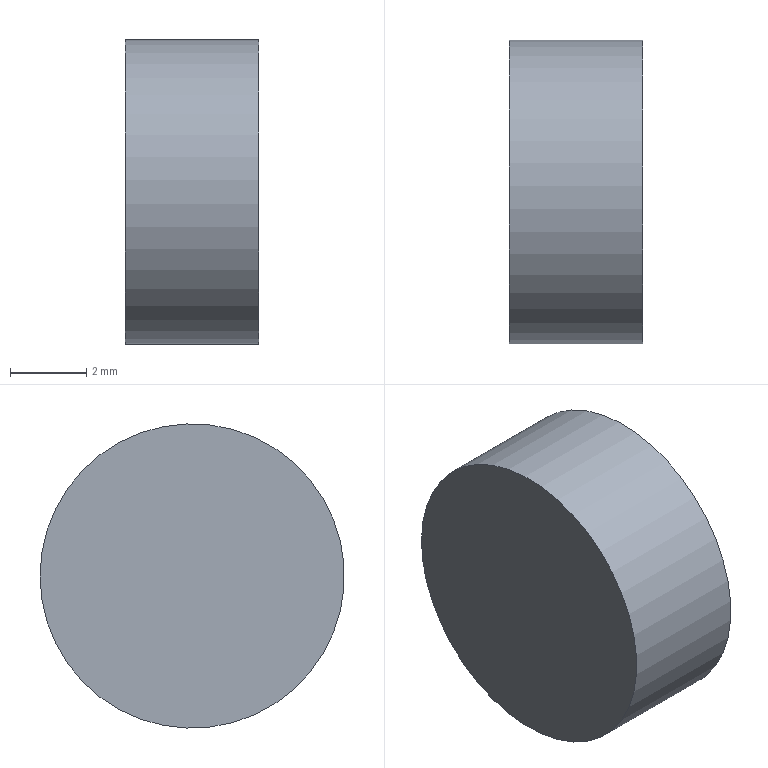Part | STEP file | 2 | 1 solid | 3 faces | box 3.5 x 8 x 8 mm | volume 175.929 mm3 | plane 2 | cylinder 1 | commonest cylinder face diameters 8 x1
STEP:
#1=CARTESIAN_POINT('',(0.,0.,0.));
#2=DIRECTION('',(0.,0.,1.));
#3=DIRECTION('',(1.,0.,0.));
#4=AXIS2_PLACEMENT_3D('',#1,#2,#3);
#5=CARTESIAN_POINT('',(-72.38,187.,0.));
#6=VERTEX_POINT('',#5);
#7=CARTESIAN_POINT('',(-72.38,183.,0.));
#8=DIRECTION('',(-1.,0.,0.));
#9=DIRECTION('',(0.,-1.,0.));
#10=AXIS2_PLACEMENT_3D('',#7,#8,#9);
#11=CIRCLE('',#10,4.);
#12=CARTESIAN_POINT('',(-70.63,183.,0.));
#13=DIRECTION('',(-1.,0.,0.));
#14=DIRECTION('',(0.,-1.,0.));
#15=AXIS2_PLACEMENT_3D('',#12,#13,#14);
#16=CYLINDRICAL_SURFACE('',#15,4.);
#17=CARTESIAN_POINT('',(0.,1.75));
#18=DIRECTION('',(1.,0.));
#19=VECTOR('',#18,1.);
#20=LINE('',#17,#19);
#21=(GEOMETRIC_REPRESENTATION_CONTEXT(2)PARAMETRIC_REPRESENTATION_CONTEXT()REPRESENTATION_CONTEXT('',''));
#22=DEFINITIONAL_REPRESENTATION('',(#20),#21);
#23=PCURVE('',#16,#22);
#24=CARTESIAN_POINT('',(-72.38,183.,0.));
#25=DIRECTION('',(-1.,0.,0.));
#26=DIRECTION('',(0.,-1.,0.));
#27=AXIS2_PLACEMENT_3D('',#24,#25,#26);
#28=PLANE('',#27);
#29=CARTESIAN_POINT('',(0.,0.));
#30=DIRECTION('',(1.,0.));
#31=AXIS2_PLACEMENT_2D('',#29,#30);
#32=CIRCLE('',#31,4.);
#33=(GEOMETRIC_REPRESENTATION_CONTEXT(2)PARAMETRIC_REPRESENTATION_CONTEXT()REPRESENTATION_CONTEXT('',''));
#34=DEFINITIONAL_REPRESENTATION('',(#32),#33);
#35=PCURVE('',#28,#34);
#36=SURFACE_CURVE('',#11,(#23,#35),.PCURVE_S1.);
#37=EDGE_CURVE('',#6,#6,#36,.T.);
#38=ORIENTED_EDGE('',*,*,#37,.F.);
#39=CARTESIAN_POINT('',(-68.88,187.,0.));
#40=VERTEX_POINT('',#39);
#41=CARTESIAN_POINT('',(-68.88,187.,0.));
#42=CARTESIAN_POINT('',(-72.38,187.,0.));
#43=B_SPLINE_CURVE_WITH_KNOTS('',1,(#41,#42),.UNSPECIFIED.,.F.,.F.,(2,2),(-1.75,1.75),.PIECEWISE_BEZIER_KNOTS.);
#44=CARTESIAN_POINT('',(3.142,0.));
#45=DIRECTION('',(0.,1.));
#46=VECTOR('',#45,1.);
#47=LINE('',#44,#46);
#48=(GEOMETRIC_REPRESENTATION_CONTEXT(2)PARAMETRIC_REPRESENTATION_CONTEXT()REPRESENTATION_CONTEXT('',''));
#49=DEFINITIONAL_REPRESENTATION('',(#47),#48);
#50=PCURVE('',#16,#49);
#51=CARTESIAN_POINT('',(9.425,0.));
#52=DIRECTION('',(0.,1.));
#53=VECTOR('',#52,1.);
#54=LINE('',#51,#53);
#55=(GEOMETRIC_REPRESENTATION_CONTEXT(2)PARAMETRIC_REPRESENTATION_CONTEXT()REPRESENTATION_CONTEXT('',''));
#56=DEFINITIONAL_REPRESENTATION('',(#54),#55);
#57=PCURVE('',#16,#56);
#58=SEAM_CURVE('',#43,(#50,#57),.PCURVE_S1.);
#59=EDGE_CURVE('',#40,#6,#58,.T.);
#60=ORIENTED_EDGE('',*,*,#59,.F.);
#61=CARTESIAN_POINT('',(-68.88,183.,0.));
#62=DIRECTION('',(1.,0.,0.));
#63=DIRECTION('',(0.,-1.,0.));
#64=AXIS2_PLACEMENT_3D('',#61,#62,#63);
#65=CIRCLE('',#64,4.);
#66=CARTESIAN_POINT('',(12.566,-1.75));
#67=DIRECTION('',(-1.,0.));
#68=VECTOR('',#67,1.);
#69=LINE('',#66,#68);
#70=(GEOMETRIC_REPRESENTATION_CONTEXT(2)PARAMETRIC_REPRESENTATION_CONTEXT()REPRESENTATION_CONTEXT('',''));
#71=DEFINITIONAL_REPRESENTATION('',(#69),#70);
#72=PCURVE('',#16,#71);
#73=CARTESIAN_POINT('',(-68.88,183.,0.));
#74=DIRECTION('',(1.,0.,0.));
#75=DIRECTION('',(0.,1.,0.));
#76=AXIS2_PLACEMENT_3D('',#73,#74,#75);
#77=PLANE('',#76);
#78=CARTESIAN_POINT('',(0.,0.));
#79=DIRECTION('',(-1.,0.));
#80=AXIS2_PLACEMENT_2D('',#78,#79);
#81=CIRCLE('',#80,4.);
#82=(GEOMETRIC_REPRESENTATION_CONTEXT(2)PARAMETRIC_REPRESENTATION_CONTEXT()REPRESENTATION_CONTEXT('',''));
#83=DEFINITIONAL_REPRESENTATION('',(#81),#82);
#84=PCURVE('',#77,#83);
#85=SURFACE_CURVE('',#65,(#72,#84),.PCURVE_S1.);
#86=EDGE_CURVE('',#40,#40,#85,.T.);
#87=ORIENTED_EDGE('',*,*,#86,.F.);
#88=ORIENTED_EDGE('',*,*,#59,.T.);
#89=EDGE_LOOP('',(#38,#60,#87,#88));
#90=FACE_BOUND('',#89,.T.);
#91=ADVANCED_FACE('',(#90),#16,.T.);
#92=ORIENTED_EDGE('',*,*,#37,.T.);
#93=EDGE_LOOP('',(#92));
#94=FACE_BOUND('',#93,.T.);
#95=ADVANCED_FACE('',(#94),#28,.T.);
#96=ORIENTED_EDGE('',*,*,#86,.T.);
#97=EDGE_LOOP('',(#96));
#98=FACE_BOUND('',#97,.T.);
#99=ADVANCED_FACE('',(#98),#77,.T.);
#100=CLOSED_SHELL('',(#91,#95,#99));
#101=MANIFOLD_SOLID_BREP('',#100);
#102=(LENGTH_UNIT()NAMED_UNIT(*)SI_UNIT(.MILLI.,.METRE.));
#103=UNCERTAINTY_MEASURE_WITH_UNIT(LENGTH_MEASURE(0.00001),#102,'','');
#104=(NAMED_UNIT(*)PLANE_ANGLE_UNIT()SI_UNIT($,.RADIAN.));
#105=(NAMED_UNIT(*)SI_UNIT($,.STERADIAN.)SOLID_ANGLE_UNIT());
#106=(GEOMETRIC_REPRESENTATION_CONTEXT(3)GLOBAL_UNCERTAINTY_ASSIGNED_CONTEXT((#103))GLOBAL_UNIT_ASSIGNED_CONTEXT((#102,#104,#105))REPRESENTATION_CONTEXT('',''));
#107=ADVANCED_BREP_SHAPE_REPRESENTATION('',(#4,#101),#106);